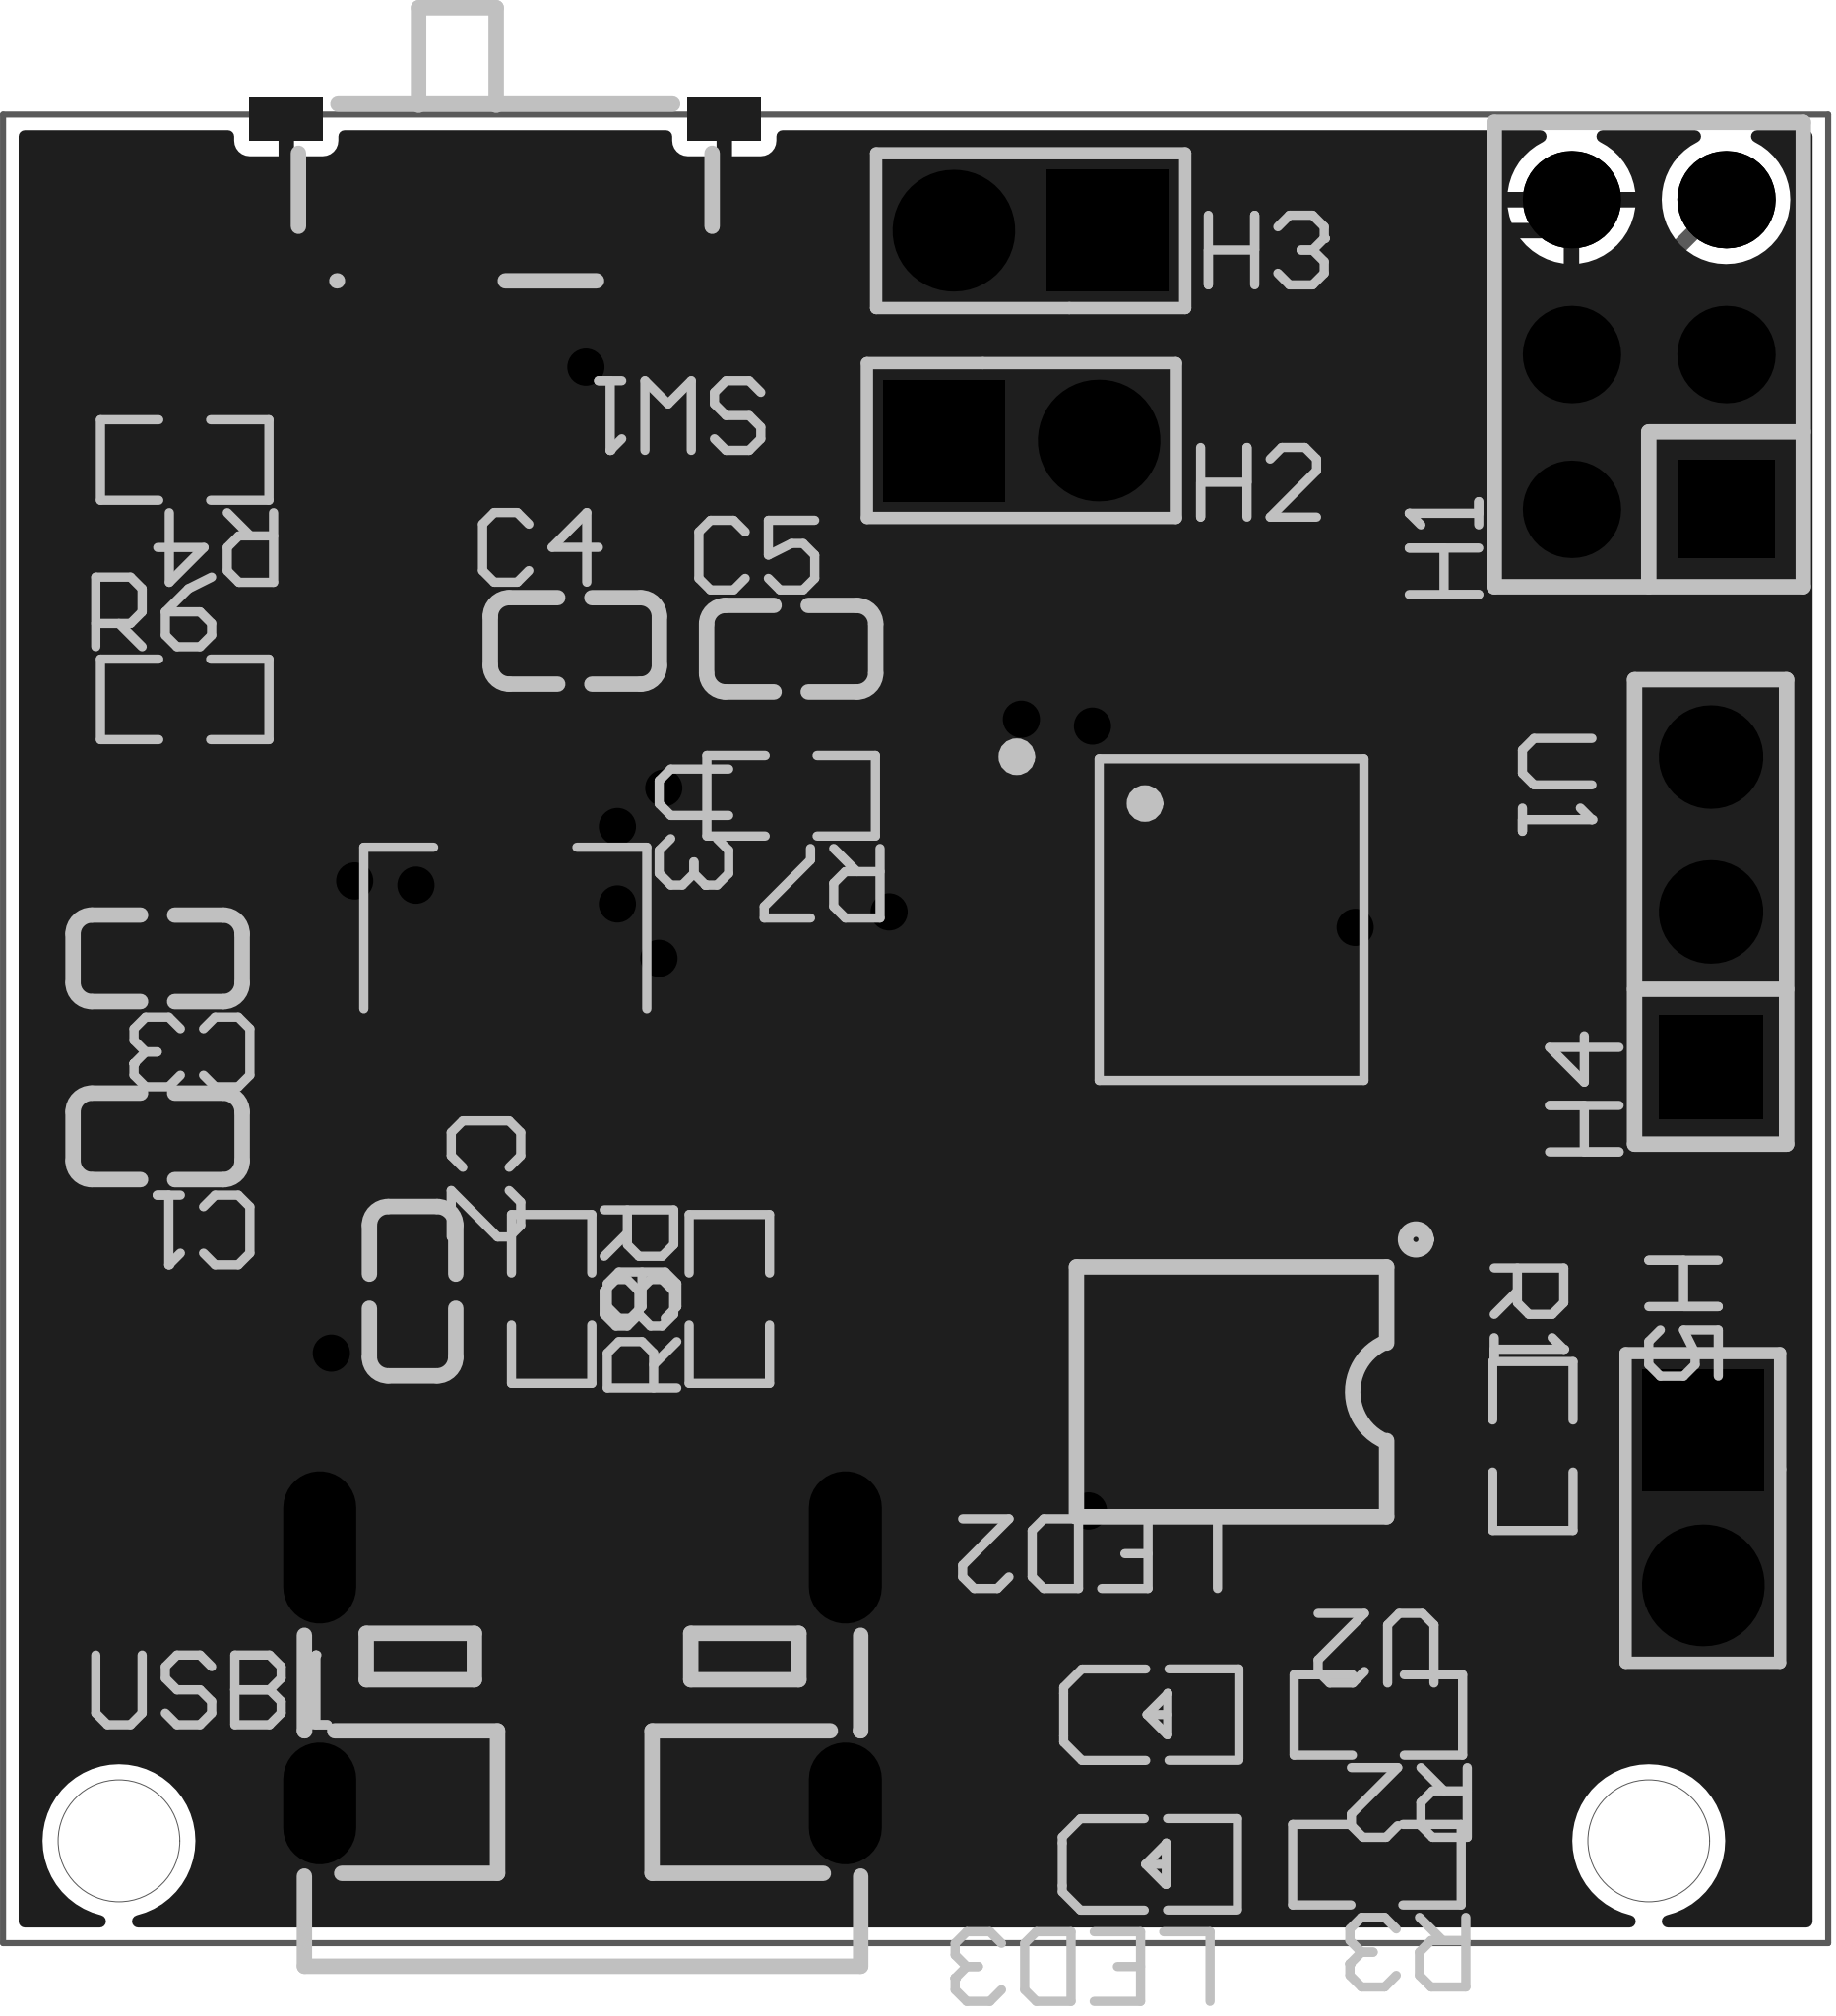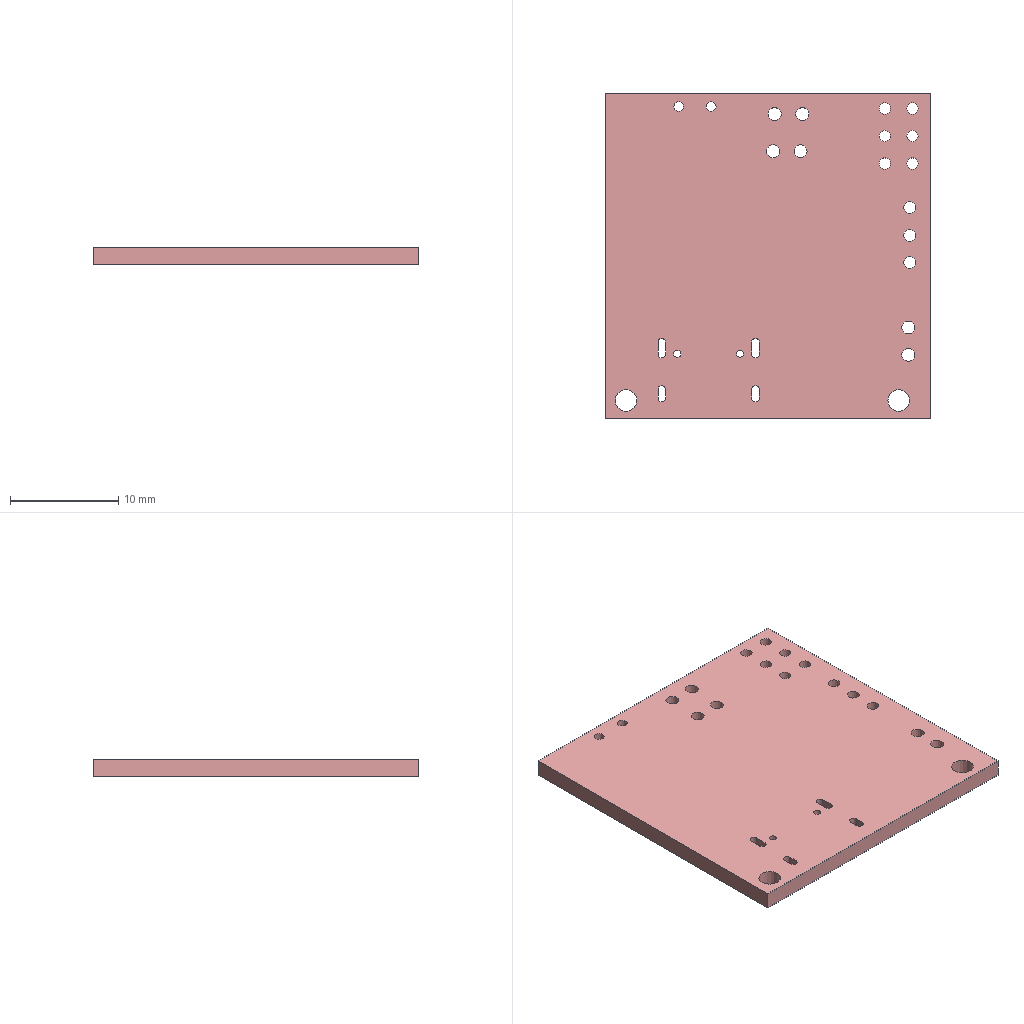Circuit board layout | Altium Designer | box 30 x 30 x 1.6 mm
Layer stack:
# Altium Designer layer stack of  (unit mm; dielectric type: 0 none, 1 core, 2 prepreg, 3 surface material)
index,name,kind,layer,copper_thickness_mm,dielectric_type,dielectric_thickness_mm,dielectric_material,dielectric_constant
0,Top Paste Mask Layer,other,,,,,,
1,Top Silkscreen Layer,other,,,,,,
2,Top Solder Mask Layer,dielectric,,,3,0.01,,3.3
3,Top Layer,copper,Top Layer,0.035,,,,
4,Dielectric1,dielectric,,,3,1.51,FR4,4.5
5,Bottom Layer,copper,Bottom Layer,0.035,,,,
6,Bottom Solder Mask Layer,dielectric,,,3,0.01,,3.3
7,Bottom Silkscreen Layer,other,,,,,,
8,Bottom Paste Mask Layer,other,,,,,,
# drill layer pairs: low layer,high layer
drill_pair,Top Layer,Bottom Layer
Part placement:
Designator,Comment,Layer,Footprint,Center-X(mm),Center-Y(mm),Rotation
C1,1uF,TopLayer,C0603,78.74,89.815,180
C2,1uF,TopLayer,C0603,82.931,87.275,270
C3,1uF,TopLayer,C0603,78.74,92.736,180
C4,1uF,TopLayer,C0603,85.598,97.943,0
C5,100nF,TopLayer,C0603,89.154,97.816,0
H1,2.54-2*3,TopLayer,HDR-TH_6P-P2.54-V-R2-C3-S2.54_A2541WV-2X3P,103.251,102.642,90
LED2,LTST-C190KSKT,TopLayer,LED0603-RD,95.123,80.322,0
LED3,LTST-C190KSKT,TopLayer,LED0603-RD,95.099,77.866,0
R1,10kΩ,TopLayer,R0603,101.346,84.735,90
R2,1kΩ,TopLayer,R0603,98.806,80.322,180
R3,1kΩ,TopLayer,R0603,98.782,77.866,180
R4,10kΩ,TopLayer,R0603,79.185,100.911,180
H2,PZ254V-11-02P,TopLayer,HDR-TH_2P-P2.54-V-M,92.939,101.23,0
R6,10kΩ,TopLayer,R0603,79.185,96.984,0
R7,10kΩ,TopLayer,R0603,89.154,95.403,180
R8,5.1kΩ,TopLayer,R0603,85.217,87.148,270
R9,5.1kΩ,TopLayer,R0603,88.138,87.148,90
SW1,MSK12C02,TopLayer,SW-TH_MSK12C02,84.455,104.801,180
H3,PZ254V-11-02P,TopLayer,HDR-TH_2P-P2.54-V-M,93.091,104.674,180
U1,ATTINY85-20SU,TopLayer,SOIC-8_L5.3-W5.3-P1.27-LS8.0-BL,96.393,93.371,270
U2,TC4056A.,TopLayer,ESOP-8_L4.9-W3.9-P1.27-LS6.0-BL-EP,96.393,85.624,180
U3,HT7333-A,TopLayer,SOT-89-3_L4.5-W2.5-P1.50-LS4.2-BR,84.455,92.414,270
USB1,MC-107D,TopLayer,USB-C-SMD_MC-107D,85.725,81.179,0
H4,PZ254V-11-03P,TopLayer,HDR-TH_3P-P2.54-V-M,104.267,93.498,90
H5,PZ254V-11-02P,TopLayer,HDR-TH_2P-P2.54-V-M,104.14,83.719,270
Pad and via stacks:
# Altium Designer via and pad stacks of  (unit mm). Each distinct definition once, with the count of objects using it.
# via: kind,start_layer,end_layer,hole_mm,diameter_mm,mode(0 simple;1 top-mid-bottom;2 full stack),diameter_per_layer,count,example_net
# pad: kind,layer,hole_mm,hole_type(0 round;1 square;2 slot),plating,top_size,top_shape(1 round;2 rect;3 octagon;9 rounded rect),mid_size,bottom_size,mode,footprint,size_per_layer,count,example
pad,Top Layer,0,0,plated,0.8x0.9,2,0.8x0.9,0.8x0.9,0,C0603,,10,C1.2
pad,Top Layer,0,0,plated,0.8x0.8,2,0.8x0.8,0.8x0.8,0,LED0603-RD,,4,LED2.2
pad,Top Layer,0,0,plated,0.8065x0.864,2,0.8065x0.864,0.8065x0.864,0,R0603,,16,R1.2
pad,Top Layer,0,0,plated,1.2x0.7,2,1.2x0.7,1.2x0.7,0,SW-TH_MSK12C02,,4,SW1.4
pad,Top Layer,0,0,plated,1.524x0.6,2,1.524x0.6,1.524x0.6,0,SW-TH_MSK12C02,,3,SW1.3
pad,Top Layer,0,0,plated,0.63x2.25,1,0.63x2.25,0.63x2.25,0,SOIC-8_L5.3-W5.3-P1.27-LS8.0-BL,,8,U1.1
pad,Top Layer,0,0,plated,0.6x1.2,2,0.6x1.2,0.6x1.2,0,ESOP-8_L4.9-W3.9-P1.27-LS6.0-BL-EP,,8,U2.1
pad,Top Layer,0,0,plated,3.3x2.4,2,3.3x2.4,3.3x2.4,0,ESOP-8_L4.9-W3.9-P1.27-LS6.0-BL-EP,,1,U2.9
pad,Top Layer,0,0,plated,1.575x0.672,2,1.575x0.672,1.575x0.672,0,SOT-89-3_L4.5-W2.5-P1.50-LS4.2-BR,,2,U3.1
pad,Top Layer,0,0,plated,0.95x0.95,1,0.95x0.95,0.95x0.95,0,SOT-89-3_L4.5-W2.5-P1.50-LS4.2-BR,,1,U3.2
pad,Top Layer,0,0,plated,0.6x1.2,2,0.6x1.2,0.6x1.2,0,USB-C-SMD_MC-107D,,4,USB1.A1B12
pad,Top Layer,0,0,plated,0.3x1.2,2,0.3x1.2,0.3x1.2,0,USB-C-SMD_MC-107D,,8,USB1.B5
pad,Multi-Layer,1.05,0,plated,1.6x1.6,2,1.6x1.6,1.6x1.6,0,HDR-TH_6P-P2.54-V-R2-C3-S2.54_A2541WV-2X3P,,1,H1.1
pad,Multi-Layer,1.05,0,plated,1.6x1.6,1,1.6x1.6,1.6x1.6,0,HDR-TH_6P-P2.54-V-R2-C3-S2.54_A2541WV-2X3P,,5,H1.2
pad,Multi-Layer,1.2,0,plated,2x2,2,2x2,2x2,0,HDR-TH_2P-P2.54-V-M,,3,H2.1
pad,Multi-Layer,1.2,0,plated,2x2,1,2x2,2x2,0,HDR-TH_2P-P2.54-V-M,,3,H2.2
pad,Multi-Layer,0.7,2,plated,1.2x2.5,1,1.2x2.5,1.2x2.5,0,USB-C-SMD_MC-107D,,2,USB1.0
pad,Multi-Layer,0.7,2,plated,1.2x2,1,1.2x2,1.2x2,0,USB-C-SMD_MC-107D,,2,USB1.0
pad,Multi-Layer,1.1,0,plated,1.7x1.7,2,1.7x1.7,1.7x1.7,0,HDR-TH_3P-P2.54-V-M,,1,H4.1
pad,Multi-Layer,1.1,0,plated,1.7x1.7,1,1.7x1.7,1.7x1.7,0,HDR-TH_3P-P2.54-V-M,,2,H4.2
via,Top Layer,Bottom Layer,0.3048,0.61,0,,13,$1N2613
Copper pours:
name,layer,net,type(0 solid;1 hatched;2 none)
Top Layer-GND,Top Layer,GND,0